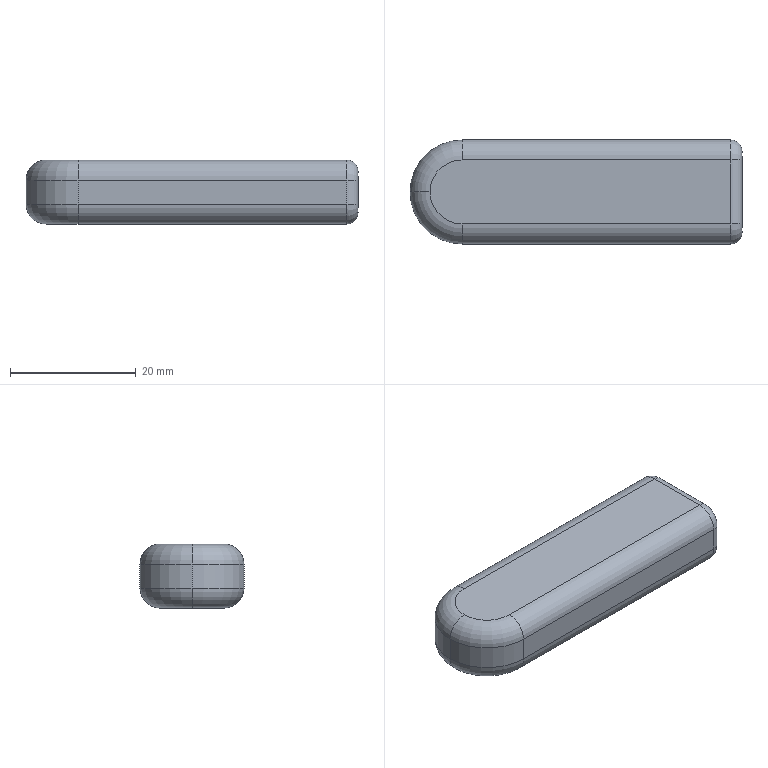Part | SolidWorks | features Fillet 3, Extrusion 1, Shell 1 | 1 solid | 32 faces | box 52.705 x 16.51 x 10.16 mm | volume 4039 mm3 | plane 12 | cylinder 12 | torus 8 | commonest cylinder face diameters 3.556 x4 6.35 x4 12.7 x2 16.51 x2
STEP:
#1=CARTESIAN_POINT('',(2.,0.05,-0.005));
#2=VERTEX_POINT('',#1);
#3=CARTESIAN_POINT('',(2.,0.45,-0.005));
#4=VERTEX_POINT('',#3);
#5=CARTESIAN_POINT('',(2.,0.5,-0.005));
#6=DIRECTION('',(0.,1.,0.));
#7=VECTOR('',#6,39.37);
#8=LINE('',#5,#7);
#9=EDGE_CURVE('',#2,#4,#8,.T.);
#10=ORIENTED_EDGE('',*,*,#9,.T.);
#11=CARTESIAN_POINT('',(2.,0.4729,0.));
#12=VERTEX_POINT('',#11);
#13=CARTESIAN_POINT('',(2.,0.45,0.05));
#14=DIRECTION('',(1.,0.,0.));
#15=DIRECTION('',(0.,0.,-1.));
#16=AXIS2_PLACEMENT_3D('',#13,#14,#15);
#17=CIRCLE('',#16,0.055);
#18=EDGE_CURVE('',#4,#12,#17,.T.);
#19=ORIENTED_EDGE('',*,*,#18,.T.);
#20=CARTESIAN_POINT('',(2.,0.02709,0.));
#21=VERTEX_POINT('',#20);
#22=CARTESIAN_POINT('',(2.,0.5,0.));
#23=DIRECTION('',(0.,-1.,0.));
#24=VECTOR('',#23,39.37);
#25=LINE('',#22,#24);
#26=EDGE_CURVE('',#12,#21,#25,.T.);
#27=ORIENTED_EDGE('',*,*,#26,.T.);
#28=CARTESIAN_POINT('',(2.,0.05,0.05));
#29=DIRECTION('',(1.,0.,0.));
#30=DIRECTION('',(0.,0.,-1.));
#31=AXIS2_PLACEMENT_3D('',#28,#29,#30);
#32=CIRCLE('',#31,0.055);
#33=EDGE_CURVE('',#21,#2,#32,.T.);
#34=ORIENTED_EDGE('',*,*,#33,.T.);
#35=EDGE_LOOP('',(#10,#19,#27,#34));
#36=FACE_OUTER_BOUND('',#35,.T.);
#37=CARTESIAN_POINT('',(2.,0.5,0.25));
#38=DIRECTION('',(1.,0.,0.));
#39=DIRECTION('',(0.,0.,-1.));
#40=AXIS2_PLACEMENT_3D('',#37,#38,#39);
#41=PLANE('',#40);
#42=ADVANCED_FACE('',(#36),#41,.T.);
#43=CARTESIAN_POINT('',(2.,0.5,0.2229));
#44=VERTEX_POINT('',#43);
#45=CARTESIAN_POINT('',(2.,0.5,0.02709));
#46=VERTEX_POINT('',#45);
#47=CARTESIAN_POINT('',(2.,0.5,0.25));
#48=DIRECTION('',(0.,0.,-1.));
#49=VECTOR('',#48,39.37);
#50=LINE('',#47,#49);
#51=EDGE_CURVE('',#44,#46,#50,.T.);
#52=ORIENTED_EDGE('',*,*,#51,.T.);
#53=CARTESIAN_POINT('',(2.,0.505,0.05));
#54=VERTEX_POINT('',#53);
#55=CARTESIAN_POINT('',(2.,0.45,0.05));
#56=DIRECTION('',(1.,0.,0.));
#57=DIRECTION('',(0.,0.,-1.));
#58=AXIS2_PLACEMENT_3D('',#55,#56,#57);
#59=CIRCLE('',#58,0.055);
#60=EDGE_CURVE('',#46,#54,#59,.T.);
#61=ORIENTED_EDGE('',*,*,#60,.T.);
#62=CARTESIAN_POINT('',(2.,0.505,0.2));
#63=VERTEX_POINT('',#62);
#64=CARTESIAN_POINT('',(2.,0.505,0.2));
#65=DIRECTION('',(0.,0.,1.));
#66=VECTOR('',#65,39.37);
#67=LINE('',#64,#66);
#68=EDGE_CURVE('',#54,#63,#67,.T.);
#69=ORIENTED_EDGE('',*,*,#68,.T.);
#70=CARTESIAN_POINT('',(2.,0.45,0.2));
#71=DIRECTION('',(1.,0.,0.));
#72=DIRECTION('',(0.,0.,-1.));
#73=AXIS2_PLACEMENT_3D('',#70,#71,#72);
#74=CIRCLE('',#73,0.055);
#75=EDGE_CURVE('',#63,#44,#74,.T.);
#76=ORIENTED_EDGE('',*,*,#75,.T.);
#77=EDGE_LOOP('',(#52,#61,#69,#76));
#78=FACE_OUTER_BOUND('',#77,.T.);
#79=CARTESIAN_POINT('',(2.,0.5,0.25));
#80=DIRECTION('',(1.,0.,0.));
#81=DIRECTION('',(0.,0.,-1.));
#82=AXIS2_PLACEMENT_3D('',#79,#80,#81);
#83=PLANE('',#82);
#84=ADVANCED_FACE('',(#78),#83,.T.);
#85=CARTESIAN_POINT('',(2.,-0.005,0.2));
#86=VERTEX_POINT('',#85);
#87=CARTESIAN_POINT('',(2.,-0.005,0.05));
#88=VERTEX_POINT('',#87);
#89=CARTESIAN_POINT('',(2.,-0.005,0.05));
#90=DIRECTION('',(0.,0.,-1.));
#91=VECTOR('',#90,39.37);
#92=LINE('',#89,#91);
#93=EDGE_CURVE('',#86,#88,#92,.T.);
#94=ORIENTED_EDGE('',*,*,#93,.T.);
#95=CARTESIAN_POINT('',(2.,0.,0.02709));
#96=VERTEX_POINT('',#95);
#97=CARTESIAN_POINT('',(2.,0.05,0.05));
#98=DIRECTION('',(1.,0.,0.));
#99=DIRECTION('',(0.,0.,-1.));
#100=AXIS2_PLACEMENT_3D('',#97,#98,#99);
#101=CIRCLE('',#100,0.055);
#102=EDGE_CURVE('',#88,#96,#101,.T.);
#103=ORIENTED_EDGE('',*,*,#102,.T.);
#104=CARTESIAN_POINT('',(2.,0.,0.2229));
#105=VERTEX_POINT('',#104);
#106=CARTESIAN_POINT('',(2.,0.,0.25));
#107=DIRECTION('',(0.,0.,-1.));
#108=VECTOR('',#107,39.37);
#109=LINE('',#106,#108);
#110=EDGE_CURVE('',#105,#96,#109,.T.);
#111=ORIENTED_EDGE('',*,*,#110,.F.);
#112=CARTESIAN_POINT('',(2.,0.05,0.2));
#113=DIRECTION('',(1.,0.,0.));
#114=DIRECTION('',(0.,0.,-1.));
#115=AXIS2_PLACEMENT_3D('',#112,#113,#114);
#116=CIRCLE('',#115,0.055);
#117=EDGE_CURVE('',#105,#86,#116,.T.);
#118=ORIENTED_EDGE('',*,*,#117,.T.);
#119=EDGE_LOOP('',(#94,#103,#111,#118));
#120=FACE_OUTER_BOUND('',#119,.T.);
#121=CARTESIAN_POINT('',(2.,0.5,0.25));
#122=DIRECTION('',(1.,0.,0.));
#123=DIRECTION('',(0.,0.,-1.));
#124=AXIS2_PLACEMENT_3D('',#121,#122,#123);
#125=PLANE('',#124);
#126=ADVANCED_FACE('',(#120),#125,.T.);
#127=CARTESIAN_POINT('',(2.,0.4729,0.25));
#128=VERTEX_POINT('',#127);
#129=CARTESIAN_POINT('',(2.,0.02709,0.25));
#130=VERTEX_POINT('',#129);
#131=CARTESIAN_POINT('',(2.,0.5,0.25));
#132=DIRECTION('',(0.,-1.,0.));
#133=VECTOR('',#132,39.37);
#134=LINE('',#131,#133);
#135=EDGE_CURVE('',#128,#130,#134,.T.);
#136=ORIENTED_EDGE('',*,*,#135,.F.);
#137=CARTESIAN_POINT('',(2.,0.45,0.255));
#138=VERTEX_POINT('',#137);
#139=CARTESIAN_POINT('',(2.,0.45,0.2));
#140=DIRECTION('',(1.,0.,0.));
#141=DIRECTION('',(0.,0.,-1.));
#142=AXIS2_PLACEMENT_3D('',#139,#140,#141);
#143=CIRCLE('',#142,0.055);
#144=EDGE_CURVE('',#128,#138,#143,.T.);
#145=ORIENTED_EDGE('',*,*,#144,.T.);
#146=CARTESIAN_POINT('',(2.,0.05,0.255));
#147=VERTEX_POINT('',#146);
#148=CARTESIAN_POINT('',(2.,0.05,0.255));
#149=DIRECTION('',(0.,-1.,0.));
#150=VECTOR('',#149,39.37);
#151=LINE('',#148,#150);
#152=EDGE_CURVE('',#138,#147,#151,.T.);
#153=ORIENTED_EDGE('',*,*,#152,.T.);
#154=CARTESIAN_POINT('',(2.,0.05,0.2));
#155=DIRECTION('',(1.,0.,0.));
#156=DIRECTION('',(0.,0.,-1.));
#157=AXIS2_PLACEMENT_3D('',#154,#155,#156);
#158=CIRCLE('',#157,0.055);
#159=EDGE_CURVE('',#147,#130,#158,.T.);
#160=ORIENTED_EDGE('',*,*,#159,.T.);
#161=EDGE_LOOP('',(#136,#145,#153,#160));
#162=FACE_OUTER_BOUND('',#161,.T.);
#163=CARTESIAN_POINT('',(2.,0.5,0.25));
#164=DIRECTION('',(1.,0.,0.));
#165=DIRECTION('',(0.,0.,-1.));
#166=AXIS2_PLACEMENT_3D('',#163,#164,#165);
#167=PLANE('',#166);
#168=ADVANCED_FACE('',(#162),#167,.T.);
#169=CARTESIAN_POINT('',(0.25,-0.075,0.05));
#170=VERTEX_POINT('',#169);
#171=CARTESIAN_POINT('',(1.93,-0.075,0.05));
#172=VERTEX_POINT('',#171);
#173=CARTESIAN_POINT('',(2.,-0.075,0.05));
#174=DIRECTION('',(1.,0.,0.));
#175=VECTOR('',#174,39.37);
#176=LINE('',#173,#175);
#177=EDGE_CURVE('',#170,#172,#176,.T.);
#178=ORIENTED_EDGE('',*,*,#177,.T.);
#179=CARTESIAN_POINT('',(1.93,-0.075,0.2));
#180=VERTEX_POINT('',#179);
#181=CARTESIAN_POINT('',(1.93,-0.075,0.2));
#182=DIRECTION('',(0.,0.,1.));
#183=VECTOR('',#182,39.37);
#184=LINE('',#181,#183);
#185=EDGE_CURVE('',#172,#180,#184,.T.);
#186=ORIENTED_EDGE('',*,*,#185,.T.);
#187=CARTESIAN_POINT('',(0.25,-0.075,0.2));
#188=VERTEX_POINT('',#187);
#189=CARTESIAN_POINT('',(0.,-0.075,0.2));
#190=DIRECTION('',(-1.,0.,0.));
#191=VECTOR('',#190,39.37);
#192=LINE('',#189,#191);
#193=EDGE_CURVE('',#180,#188,#192,.T.);
#194=ORIENTED_EDGE('',*,*,#193,.T.);
#195=CARTESIAN_POINT('',(0.25,-0.075,0.25));
#196=DIRECTION('',(0.,0.,-1.));
#197=VECTOR('',#196,39.37);
#198=LINE('',#195,#197);
#199=EDGE_CURVE('',#188,#170,#198,.T.);
#200=ORIENTED_EDGE('',*,*,#199,.T.);
#201=EDGE_LOOP('',(#178,#186,#194,#200));
#202=FACE_OUTER_BOUND('',#201,.T.);
#203=CARTESIAN_POINT('',(0.,-0.075,0.25));
#204=DIRECTION('',(0.,1.,0.));
#205=DIRECTION('',(0.,0.,1.));
#206=AXIS2_PLACEMENT_3D('',#203,#204,#205);
#207=PLANE('',#206);
#208=ADVANCED_FACE('',(#202),#207,.F.);
#209=CARTESIAN_POINT('',(0.25,0.575,0.2));
#210=VERTEX_POINT('',#209);
#211=CARTESIAN_POINT('',(1.93,0.575,0.2));
#212=VERTEX_POINT('',#211);
#213=CARTESIAN_POINT('',(2.,0.575,0.2));
#214=DIRECTION('',(1.,0.,0.));
#215=VECTOR('',#214,39.37);
#216=LINE('',#213,#215);
#217=EDGE_CURVE('',#210,#212,#216,.T.);
#218=ORIENTED_EDGE('',*,*,#217,.T.);
#219=CARTESIAN_POINT('',(1.93,0.575,0.05));
#220=VERTEX_POINT('',#219);
#221=CARTESIAN_POINT('',(1.93,0.575,0.05));
#222=DIRECTION('',(0.,0.,-1.));
#223=VECTOR('',#222,39.37);
#224=LINE('',#221,#223);
#225=EDGE_CURVE('',#212,#220,#224,.T.);
#226=ORIENTED_EDGE('',*,*,#225,.T.);
#227=CARTESIAN_POINT('',(0.25,0.575,0.05));
#228=VERTEX_POINT('',#227);
#229=CARTESIAN_POINT('',(0.25,0.575,0.05));
#230=DIRECTION('',(-1.,0.,0.));
#231=VECTOR('',#230,39.37);
#232=LINE('',#229,#231);
#233=EDGE_CURVE('',#220,#228,#232,.T.);
#234=ORIENTED_EDGE('',*,*,#233,.T.);
#235=CARTESIAN_POINT('',(0.25,0.575,0.25));
#236=DIRECTION('',(0.,0.,1.));
#237=VECTOR('',#236,39.37);
#238=LINE('',#235,#237);
#239=EDGE_CURVE('',#228,#210,#238,.T.);
#240=ORIENTED_EDGE('',*,*,#239,.T.);
#241=EDGE_LOOP('',(#218,#226,#234,#240));
#242=FACE_OUTER_BOUND('',#241,.T.);
#243=CARTESIAN_POINT('',(2.,0.575,0.25));
#244=DIRECTION('',(0.,-1.,0.));
#245=DIRECTION('',(1.,0.,0.));
#246=AXIS2_PLACEMENT_3D('',#243,#244,#245);
#247=PLANE('',#246);
#248=ADVANCED_FACE('',(#242),#247,.F.);
#249=CARTESIAN_POINT('',(0.25,0.05,0.325));
#250=VERTEX_POINT('',#249);
#251=CARTESIAN_POINT('',(1.93,0.05,0.325));
#252=VERTEX_POINT('',#251);
#253=CARTESIAN_POINT('',(0.,0.05,0.325));
#254=DIRECTION('',(1.,0.,0.));
#255=VECTOR('',#254,39.37);
#256=LINE('',#253,#255);
#257=EDGE_CURVE('',#250,#252,#256,.T.);
#258=ORIENTED_EDGE('',*,*,#257,.T.);
#259=CARTESIAN_POINT('',(1.93,0.45,0.325));
#260=VERTEX_POINT('',#259);
#261=CARTESIAN_POINT('',(1.93,0.45,0.325));
#262=DIRECTION('',(0.,1.,0.));
#263=VECTOR('',#262,39.37);
#264=LINE('',#261,#263);
#265=EDGE_CURVE('',#252,#260,#264,.T.);
#266=ORIENTED_EDGE('',*,*,#265,.T.);
#267=CARTESIAN_POINT('',(0.25,0.45,0.325));
#268=VERTEX_POINT('',#267);
#269=CARTESIAN_POINT('',(0.,0.45,0.325));
#270=DIRECTION('',(-1.,0.,0.));
#271=VECTOR('',#270,39.37);
#272=LINE('',#269,#271);
#273=EDGE_CURVE('',#260,#268,#272,.T.);
#274=ORIENTED_EDGE('',*,*,#273,.T.);
#275=CARTESIAN_POINT('',(0.05,0.25,0.325));
#276=VERTEX_POINT('',#275);
#277=CARTESIAN_POINT('',(0.25,0.25,0.325));
#278=DIRECTION('',(0.,0.,1.));
#279=DIRECTION('',(-1.,0.,0.));
#280=AXIS2_PLACEMENT_3D('',#277,#278,#279);
#281=CIRCLE('',#280,0.2);
#282=EDGE_CURVE('',#268,#276,#281,.T.);
#283=ORIENTED_EDGE('',*,*,#282,.T.);
#284=CARTESIAN_POINT('',(0.25,0.25,0.325));
#285=DIRECTION('',(0.,0.,1.));
#286=DIRECTION('',(-1.,0.,0.));
#287=AXIS2_PLACEMENT_3D('',#284,#285,#286);
#288=CIRCLE('',#287,0.2);
#289=EDGE_CURVE('',#276,#250,#288,.T.);
#290=ORIENTED_EDGE('',*,*,#289,.T.);
#291=EDGE_LOOP('',(#258,#266,#274,#283,#290));
#292=FACE_OUTER_BOUND('',#291,.T.);
#293=CARTESIAN_POINT('',(0.,0.,0.325));
#294=DIRECTION('',(0.,0.,-1.));
#295=DIRECTION('',(-1.,0.,0.));
#296=AXIS2_PLACEMENT_3D('',#293,#294,#295);
#297=PLANE('',#296);
#298=ADVANCED_FACE('',(#292),#297,.F.);
#299=CARTESIAN_POINT('',(0.25,0.45,-0.075));
#300=VERTEX_POINT('',#299);
#301=CARTESIAN_POINT('',(1.93,0.45,-0.075));
#302=VERTEX_POINT('',#301);
#303=CARTESIAN_POINT('',(2.,0.45,-0.075));
#304=DIRECTION('',(1.,0.,0.));
#305=VECTOR('',#304,39.37);
#306=LINE('',#303,#305);
#307=EDGE_CURVE('',#300,#302,#306,.T.);
#308=ORIENTED_EDGE('',*,*,#307,.T.);
#309=CARTESIAN_POINT('',(1.93,0.05,-0.075));
#310=VERTEX_POINT('',#309);
#311=CARTESIAN_POINT('',(1.93,0.,-0.075));
#312=DIRECTION('',(0.,-1.,0.));
#313=VECTOR('',#312,39.37);
#314=LINE('',#311,#313);
#315=EDGE_CURVE('',#302,#310,#314,.T.);
#316=ORIENTED_EDGE('',*,*,#315,.T.);
#317=CARTESIAN_POINT('',(0.25,0.05,-0.075));
#318=VERTEX_POINT('',#317);
#319=CARTESIAN_POINT('',(0.25,0.05,-0.075));
#320=DIRECTION('',(-1.,0.,0.));
#321=VECTOR('',#320,39.37);
#322=LINE('',#319,#321);
#323=EDGE_CURVE('',#310,#318,#322,.T.);
#324=ORIENTED_EDGE('',*,*,#323,.T.);
#325=CARTESIAN_POINT('',(0.05,0.25,-0.075));
#326=VERTEX_POINT('',#325);
#327=CARTESIAN_POINT('',(0.25,0.25,-0.075));
#328=DIRECTION('',(0.,0.,-1.));
#329=DIRECTION('',(-1.,0.,0.));
#330=AXIS2_PLACEMENT_3D('',#327,#328,#329);
#331=CIRCLE('',#330,0.2);
#332=EDGE_CURVE('',#318,#326,#331,.T.);
#333=ORIENTED_EDGE('',*,*,#332,.T.);
#334=CARTESIAN_POINT('',(0.25,0.25,-0.075));
#335=DIRECTION('',(0.,0.,-1.));
#336=DIRECTION('',(-1.,0.,0.));
#337=AXIS2_PLACEMENT_3D('',#334,#335,#336);
#338=CIRCLE('',#337,0.2);
#339=EDGE_CURVE('',#326,#300,#338,.T.);
#340=ORIENTED_EDGE('',*,*,#339,.T.);
#341=EDGE_LOOP('',(#308,#316,#324,#333,#340));
#342=FACE_OUTER_BOUND('',#341,.T.);
#343=CARTESIAN_POINT('',(0.,0.,-0.075));
#344=DIRECTION('',(0.,0.,-1.));
#345=DIRECTION('',(-1.,0.,0.));
#346=AXIS2_PLACEMENT_3D('',#343,#344,#345);
#347=PLANE('',#346);
#348=ADVANCED_FACE('',(#342),#347,.T.);
#349=CARTESIAN_POINT('',(-0.075,0.25,0.05));
#350=VERTEX_POINT('',#349);
#351=CARTESIAN_POINT('',(-0.075,0.25,0.2));
#352=VERTEX_POINT('',#351);
#353=CARTESIAN_POINT('',(-0.075,0.25,0.25));
#354=DIRECTION('',(0.,0.,1.));
#355=VECTOR('',#354,39.37);
#356=LINE('',#353,#355);
#357=EDGE_CURVE('',#350,#352,#356,.T.);
#358=ORIENTED_EDGE('',*,*,#357,.F.);
#359=CARTESIAN_POINT('',(0.25,0.25,0.05));
#360=DIRECTION('',(0.,0.,1.));
#361=DIRECTION('',(-1.,0.,0.));
#362=AXIS2_PLACEMENT_3D('',#359,#360,#361);
#363=CIRCLE('',#362,0.325);
#364=EDGE_CURVE('',#350,#170,#363,.T.);
#365=ORIENTED_EDGE('',*,*,#364,.T.);
#366=ORIENTED_EDGE('',*,*,#199,.F.);
#367=CARTESIAN_POINT('',(0.25,0.25,0.2));
#368=DIRECTION('',(0.,0.,-1.));
#369=DIRECTION('',(-1.,0.,0.));
#370=AXIS2_PLACEMENT_3D('',#367,#368,#369);
#371=CIRCLE('',#370,0.325);
#372=EDGE_CURVE('',#188,#352,#371,.T.);
#373=ORIENTED_EDGE('',*,*,#372,.T.);
#374=EDGE_LOOP('',(#358,#365,#366,#373));
#375=FACE_OUTER_BOUND('',#374,.T.);
#376=CARTESIAN_POINT('',(0.25,0.25,0.25));
#377=DIRECTION('',(0.,0.,1.));
#378=DIRECTION('',(1.,0.,0.));
#379=AXIS2_PLACEMENT_3D('',#376,#377,#378);
#380=CYLINDRICAL_SURFACE('',#379,0.325);
#381=ADVANCED_FACE('',(#375),#380,.T.);
#382=ORIENTED_EDGE('',*,*,#239,.F.);
#383=CARTESIAN_POINT('',(0.25,0.25,0.05));
#384=DIRECTION('',(0.,0.,1.));
#385=DIRECTION('',(-1.,0.,0.));
#386=AXIS2_PLACEMENT_3D('',#383,#384,#385);
#387=CIRCLE('',#386,0.325);
#388=EDGE_CURVE('',#228,#350,#387,.T.);
#389=ORIENTED_EDGE('',*,*,#388,.T.);
#390=ORIENTED_EDGE('',*,*,#357,.T.);
#391=CARTESIAN_POINT('',(0.25,0.25,0.2));
#392=DIRECTION('',(0.,0.,-1.));
#393=DIRECTION('',(-1.,0.,0.));
#394=AXIS2_PLACEMENT_3D('',#391,#392,#393);
#395=CIRCLE('',#394,0.325);
#396=EDGE_CURVE('',#352,#210,#395,.T.);
#397=ORIENTED_EDGE('',*,*,#396,.T.);
#398=EDGE_LOOP('',(#382,#389,#390,#397));
#399=FACE_OUTER_BOUND('',#398,.T.);
#400=CARTESIAN_POINT('',(0.25,0.25,0.25));
#401=DIRECTION('',(0.,0.,1.));
#402=DIRECTION('',(1.,0.,0.));
#403=AXIS2_PLACEMENT_3D('',#400,#401,#402);
#404=CYLINDRICAL_SURFACE('',#403,0.325);
#405=ADVANCED_FACE('',(#399),#404,.T.);
#406=ORIENTED_EDGE('',*,*,#110,.T.);
#407=CARTESIAN_POINT('',(1.998,0.,0.));
#408=VERTEX_POINT('',#407);
#409=CARTESIAN_POINT('',(2.,0.,0.02709));
#410=CARTESIAN_POINT('',(2.,0.,0.01802));
#411=CARTESIAN_POINT('',(2.,0.,0.008972));
#412=CARTESIAN_POINT('',(1.998,0.,0.));
#413=B_SPLINE_CURVE_WITH_KNOTS('',3,(#409,#410,#411,#412),.UNSPECIFIED.,.F.,.F.,(4,4),(0.,0.0006895),.UNSPECIFIED.);
#414=EDGE_CURVE('',#96,#408,#413,.T.);
#415=ORIENTED_EDGE('',*,*,#414,.T.);
#416=CARTESIAN_POINT('',(0.25,0.,0.));
#417=VERTEX_POINT('',#416);
#418=CARTESIAN_POINT('',(0.,0.,0.));
#419=DIRECTION('',(1.,0.,0.));
#420=VECTOR('',#419,39.37);
#421=LINE('',#418,#420);
#422=EDGE_CURVE('',#417,#408,#421,.T.);
#423=ORIENTED_EDGE('',*,*,#422,.F.);
#424=CARTESIAN_POINT('',(0.25,0.,0.25));
#425=VERTEX_POINT('',#424);
#426=CARTESIAN_POINT('',(0.25,0.,0.));
#427=DIRECTION('',(0.,0.,-1.));
#428=VECTOR('',#427,39.37);
#429=LINE('',#426,#428);
#430=EDGE_CURVE('',#425,#417,#429,.T.);
#431=ORIENTED_EDGE('',*,*,#430,.F.);
#432=CARTESIAN_POINT('',(1.998,0.,0.25));
#433=VERTEX_POINT('',#432);
#434=CARTESIAN_POINT('',(0.,0.,0.25));
#435=DIRECTION('',(1.,0.,0.));
#436=VECTOR('',#435,39.37);
#437=LINE('',#434,#436);
#438=EDGE_CURVE('',#425,#433,#437,.T.);
#439=ORIENTED_EDGE('',*,*,#438,.T.);
#440=CARTESIAN_POINT('',(1.998,0.,0.25));
#441=CARTESIAN_POINT('',(2.,0.,0.241));
#442=CARTESIAN_POINT('',(2.,0.,0.232));
#443=CARTESIAN_POINT('',(2.,0.,0.2229));
#444=B_SPLINE_CURVE_WITH_KNOTS('',3,(#440,#441,#442,#443),.UNSPECIFIED.,.F.,.F.,(4,4),(0.,0.0006895),.UNSPECIFIED.);
#445=EDGE_CURVE('',#433,#105,#444,.T.);
#446=ORIENTED_EDGE('',*,*,#445,.T.);
#447=EDGE_LOOP('',(#406,#415,#423,#431,#439,#446));
#448=FACE_OUTER_BOUND('',#447,.T.);
#449=CARTESIAN_POINT('',(0.,0.,0.25));
#450=DIRECTION('',(0.,1.,0.));
#451=DIRECTION('',(0.,0.,1.));
#452=AXIS2_PLACEMENT_3D('',#449,#450,#451);
#453=PLANE('',#452);
#454=ADVANCED_FACE('',(#448),#453,.T.);
#455=CARTESIAN_POINT('',(1.998,0.5,0.));
#456=VERTEX_POINT('',#455);
#457=CARTESIAN_POINT('',(0.25,0.5,0.));
#458=VERTEX_POINT('',#457);
#459=CARTESIAN_POINT('',(2.,0.5,0.));
#460=DIRECTION('',(-1.,0.,0.));
#461=VECTOR('',#460,39.37);
#462=LINE('',#459,#461);
#463=EDGE_CURVE('',#456,#458,#462,.T.);
#464=ORIENTED_EDGE('',*,*,#463,.F.);
#465=CARTESIAN_POINT('',(1.998,0.5,0.));
#466=CARTESIAN_POINT('',(2.,0.5,0.008972));
#467=CARTESIAN_POINT('',(2.,0.5,0.01802));
#468=CARTESIAN_POINT('',(2.,0.5,0.02709));
#469=B_SPLINE_CURVE_WITH_KNOTS('',3,(#465,#466,#467,#468),.UNSPECIFIED.,.F.,.F.,(4,4),(0.,0.0006895),.UNSPECIFIED.);
#470=EDGE_CURVE('',#456,#46,#469,.T.);
#471=ORIENTED_EDGE('',*,*,#470,.T.);
#472=ORIENTED_EDGE('',*,*,#51,.F.);
#473=CARTESIAN_POINT('',(1.998,0.5,0.25));
#474=VERTEX_POINT('',#473);
#475=CARTESIAN_POINT('',(2.,0.5,0.2229));
#476=CARTESIAN_POINT('',(2.,0.5,0.232));
#477=CARTESIAN_POINT('',(2.,0.5,0.241));
#478=CARTESIAN_POINT('',(1.998,0.5,0.25));
#479=B_SPLINE_CURVE_WITH_KNOTS('',3,(#475,#476,#477,#478),.UNSPECIFIED.,.F.,.F.,(4,4),(0.,0.0006895),.UNSPECIFIED.);
#480=EDGE_CURVE('',#44,#474,#479,.T.);
#481=ORIENTED_EDGE('',*,*,#480,.T.);
#482=CARTESIAN_POINT('',(0.25,0.5,0.25));
#483=VERTEX_POINT('',#482);
#484=CARTESIAN_POINT('',(2.,0.5,0.25));
#485=DIRECTION('',(-1.,0.,0.));
#486=VECTOR('',#485,39.37);
#487=LINE('',#484,#486);
#488=EDGE_CURVE('',#474,#483,#487,.T.);
#489=ORIENTED_EDGE('',*,*,#488,.T.);
#490=CARTESIAN_POINT('',(0.25,0.5,0.25));
#491=DIRECTION('',(0.,0.,1.));
#492=VECTOR('',#491,39.37);
#493=LINE('',#490,#492);
#494=EDGE_CURVE('',#458,#483,#493,.T.);
#495=ORIENTED_EDGE('',*,*,#494,.F.);
#496=EDGE_LOOP('',(#464,#471,#472,#481,#489,#495));
#497=FACE_OUTER_BOUND('',#496,.T.);
#498=CARTESIAN_POINT('',(2.,0.5,0.25));
#499=DIRECTION('',(0.,-1.,0.));
#500=DIRECTION('',(1.,0.,0.));
#501=AXIS2_PLACEMENT_3D('',#498,#499,#500);
#502=PLANE('',#501);
#503=ADVANCED_FACE('',(#497),#502,.T.);
#504=ORIENTED_EDGE('',*,*,#488,.F.);
#505=CARTESIAN_POINT('',(1.998,0.5,0.25));
#506=CARTESIAN_POINT('',(2.,0.491,0.25));
#507=CARTESIAN_POINT('',(2.,0.482,0.25));
#508=CARTESIAN_POINT('',(2.,0.4729,0.25));
#509=B_SPLINE_CURVE_WITH_KNOTS('',3,(#505,#506,#507,#508),.UNSPECIFIED.,.F.,.F.,(4,4),(0.,0.0006895),.UNSPECIFIED.);
#510=EDGE_CURVE('',#474,#128,#509,.T.);
#511=ORIENTED_EDGE('',*,*,#510,.T.);
#512=ORIENTED_EDGE('',*,*,#135,.T.);
#513=CARTESIAN_POINT('',(2.,0.02709,0.25));
#514=CARTESIAN_POINT('',(2.,0.01802,0.25));
#515=CARTESIAN_POINT('',(2.,0.008972,0.25));
#516=CARTESIAN_POINT('',(1.998,0.,0.25));
#517=B_SPLINE_CURVE_WITH_KNOTS('',3,(#513,#514,#515,#516),.UNSPECIFIED.,.F.,.F.,(4,4),(0.,0.0006895),.UNSPECIFIED.);
#518=EDGE_CURVE('',#130,#433,#517,.T.);
#519=ORIENTED_EDGE('',*,*,#518,.T.);
#520=ORIENTED_EDGE('',*,*,#438,.F.);
#521=CARTESIAN_POINT('',(0.,0.25,0.25));
#522=VERTEX_POINT('',#521);
#523=CARTESIAN_POINT('',(0.25,0.25,0.25));
#524=DIRECTION('',(0.,0.,1.));
#525=DIRECTION('',(-1.,0.,0.));
#526=AXIS2_PLACEMENT_3D('',#523,#524,#525);
#527=CIRCLE('',#526,0.25);
#528=EDGE_CURVE('',#522,#425,#527,.T.);
#529=ORIENTED_EDGE('',*,*,#528,.F.);
#530=CARTESIAN_POINT('',(0.25,0.25,0.25));
#531=DIRECTION('',(0.,0.,1.));
#532=DIRECTION('',(-1.,0.,0.));
#533=AXIS2_PLACEMENT_3D('',#530,#531,#532);
#534=CIRCLE('',#533,0.25);
#535=EDGE_CURVE('',#483,#522,#534,.T.);
#536=ORIENTED_EDGE('',*,*,#535,.F.);
#537=EDGE_LOOP('',(#504,#511,#512,#519,#520,#529,#536));
#538=FACE_OUTER_BOUND('',#537,.T.);
#539=CARTESIAN_POINT('',(0.,0.,0.25));
#540=DIRECTION('',(0.,0.,-1.));
#541=DIRECTION('',(-1.,0.,0.));
#542=AXIS2_PLACEMENT_3D('',#539,#540,#541);
#543=PLANE('',#542);
#544=ADVANCED_FACE('',(#538),#543,.T.);
#545=ORIENTED_EDGE('',*,*,#26,.F.);
#546=CARTESIAN_POINT('',(2.,0.4729,0.));
#547=CARTESIAN_POINT('',(2.,0.482,0.));
#548=CARTESIAN_POINT('',(2.,0.491,0.));
#549=CARTESIAN_POINT('',(1.998,0.5,0.));
#550=B_SPLINE_CURVE_WITH_KNOTS('',3,(#546,#547,#548,#549),.UNSPECIFIED.,.F.,.F.,(4,4),(0.,0.0006895),.UNSPECIFIED.);
#551=EDGE_CURVE('',#12,#456,#550,.T.);
#552=ORIENTED_EDGE('',*,*,#551,.T.);
#553=ORIENTED_EDGE('',*,*,#463,.T.);
#554=CARTESIAN_POINT('',(0.,0.25,0.));
#555=VERTEX_POINT('',#554);
#556=CARTESIAN_POINT('',(0.25,0.25,0.));
#557=DIRECTION('',(0.,0.,-1.));
#558=DIRECTION('',(-1.,0.,0.));
#559=AXIS2_PLACEMENT_3D('',#556,#557,#558);
#560=CIRCLE('',#559,0.25);
#561=EDGE_CURVE('',#555,#458,#560,.T.);
#562=ORIENTED_EDGE('',*,*,#561,.F.);
#563=CARTESIAN_POINT('',(0.25,0.25,0.));
#564=DIRECTION('',(0.,0.,-1.));
#565=DIRECTION('',(-1.,0.,0.));
#566=AXIS2_PLACEMENT_3D('',#563,#564,#565);
#567=CIRCLE('',#566,0.25);
#568=EDGE_CURVE('',#417,#555,#567,.T.);
#569=ORIENTED_EDGE('',*,*,#568,.F.);
#570=ORIENTED_EDGE('',*,*,#422,.T.);
#571=CARTESIAN_POINT('',(1.998,0.,0.));
#572=CARTESIAN_POINT('',(2.,0.008972,0.));
#573=CARTESIAN_POINT('',(2.,0.01802,0.));
#574=CARTESIAN_POINT('',(2.,0.02709,0.));
#575=B_SPLINE_CURVE_WITH_KNOTS('',3,(#571,#572,#573,#574),.UNSPECIFIED.,.F.,.F.,(4,4),(0.,0.0006895),.UNSPECIFIED.);
#576=EDGE_CURVE('',#408,#21,#575,.T.);
#577=ORIENTED_EDGE('',*,*,#576,.T.);
#578=EDGE_LOOP('',(#545,#552,#553,#562,#569,#570,#577));
#579=FACE_OUTER_BOUND('',#578,.T.);
#580=CARTESIAN_POINT('',(0.,0.,0.));
#581=DIRECTION('',(0.,0.,-1.));
#582=DIRECTION('',(-1.,0.,0.));
#583=AXIS2_PLACEMENT_3D('',#580,#581,#582);
#584=PLANE('',#583);
#585=ADVANCED_FACE('',(#579),#584,.F.);
#586=ORIENTED_EDGE('',*,*,#430,.T.);
#587=ORIENTED_EDGE('',*,*,#568,.T.);
#588=CARTESIAN_POINT('',(0.,0.25,0.25));
#589=DIRECTION('',(0.,0.,1.));
#590=VECTOR('',#589,39.37);
#591=LINE('',#588,#590);
#592=EDGE_CURVE('',#555,#522,#591,.T.);
#593=ORIENTED_EDGE('',*,*,#592,.T.);
#594=ORIENTED_EDGE('',*,*,#528,.T.);
#595=EDGE_LOOP('',(#586,#587,#593,#594));
#596=FACE_OUTER_BOUND('',#595,.T.);
#597=CARTESIAN_POINT('',(0.25,0.25,0.25));
#598=DIRECTION('',(0.,0.,1.));
#599=DIRECTION('',(1.,0.,0.));
#600=AXIS2_PLACEMENT_3D('',#597,#598,#599);
#601=CYLINDRICAL_SURFACE('',#600,0.25);
#602=ADVANCED_FACE('',(#596),#601,.F.);
#603=ORIENTED_EDGE('',*,*,#535,.T.);
#604=ORIENTED_EDGE('',*,*,#592,.F.);
#605=ORIENTED_EDGE('',*,*,#561,.T.);
#606=ORIENTED_EDGE('',*,*,#494,.T.);
#607=EDGE_LOOP('',(#603,#604,#605,#606));
#608=FACE_OUTER_BOUND('',#607,.T.);
#609=CARTESIAN_POINT('',(0.25,0.25,0.25));
#610=DIRECTION('',(0.,0.,1.));
#611=DIRECTION('',(1.,0.,0.));
#612=AXIS2_PLACEMENT_3D('',#609,#610,#611);
#613=CYLINDRICAL_SURFACE('',#612,0.25);
#614=ADVANCED_FACE('',(#608),#613,.F.);
#615=ORIENTED_EDGE('',*,*,#233,.F.);
#616=CARTESIAN_POINT('',(1.93,0.45,0.05));
#617=DIRECTION('',(-1.,0.,0.));
#618=DIRECTION('',(0.,0.,-1.));
#619=AXIS2_PLACEMENT_3D('',#616,#617,#618);
#620=CIRCLE('',#619,0.125);
#621=EDGE_CURVE('',#220,#302,#620,.T.);
#622=ORIENTED_EDGE('',*,*,#621,.T.);
#623=ORIENTED_EDGE('',*,*,#307,.F.);
#624=CARTESIAN_POINT('',(0.25,0.45,0.05));
#625=DIRECTION('',(-1.,0.,0.));
#626=DIRECTION('',(0.,0.,1.));
#627=AXIS2_PLACEMENT_3D('',#624,#625,#626);
#628=CIRCLE('',#627,0.125);
#629=EDGE_CURVE('',#228,#300,#628,.T.);
#630=ORIENTED_EDGE('',*,*,#629,.F.);
#631=EDGE_LOOP('',(#615,#622,#623,#630));
#632=FACE_OUTER_BOUND('',#631,.T.);
#633=CARTESIAN_POINT('',(2.,0.45,0.05));
#634=DIRECTION('',(1.,0.,0.));
#635=DIRECTION('',(0.,1.,0.));
#636=AXIS2_PLACEMENT_3D('',#633,#634,#635);
#637=CYLINDRICAL_SURFACE('',#636,0.125);
#638=ADVANCED_FACE('',(#632),#637,.T.);
#639=ORIENTED_EDGE('',*,*,#629,.T.);
#640=ORIENTED_EDGE('',*,*,#339,.F.);
#641=CARTESIAN_POINT('',(0.05,0.25,0.05));
#642=DIRECTION('',(0.,-1.,0.));
#643=DIRECTION('',(0.,0.,-1.));
#644=AXIS2_PLACEMENT_3D('',#641,#642,#643);
#645=CIRCLE('',#644,0.125);
#646=EDGE_CURVE('',#350,#326,#645,.T.);
#647=ORIENTED_EDGE('',*,*,#646,.F.);
#648=ORIENTED_EDGE('',*,*,#388,.F.);
#649=EDGE_LOOP('',(#639,#640,#647,#648));
#650=FACE_OUTER_BOUND('',#649,.T.);
#651=CARTESIAN_POINT('',(0.25,0.25,0.05));
#652=DIRECTION('',(0.,0.,-1.));
#653=DIRECTION('',(-1.,0.,0.));
#654=AXIS2_PLACEMENT_3D('',#651,#652,#653);
#655=TOROIDAL_SURFACE('',#654,0.2,0.125);
#656=ADVANCED_FACE('',(#650),#655,.T.);
#657=ORIENTED_EDGE('',*,*,#646,.T.);
#658=ORIENTED_EDGE('',*,*,#332,.F.);
#659=CARTESIAN_POINT('',(0.25,0.05,0.05));
#660=DIRECTION('',(1.,0.,0.));
#661=DIRECTION('',(0.,0.,-1.));
#662=AXIS2_PLACEMENT_3D('',#659,#660,#661);
#663=CIRCLE('',#662,0.125);
#664=EDGE_CURVE('',#170,#318,#663,.T.);
#665=ORIENTED_EDGE('',*,*,#664,.F.);
#666=ORIENTED_EDGE('',*,*,#364,.F.);
#667=EDGE_LOOP('',(#657,#658,#665,#666));
#668=FACE_OUTER_BOUND('',#667,.T.);
#669=CARTESIAN_POINT('',(0.25,0.25,0.05));
#670=DIRECTION('',(0.,0.,-1.));
#671=DIRECTION('',(-1.,0.,0.));
#672=AXIS2_PLACEMENT_3D('',#669,#670,#671);
#673=TOROIDAL_SURFACE('',#672,0.2,0.125);
#674=ADVANCED_FACE('',(#668),#673,.T.);
#675=ORIENTED_EDGE('',*,*,#323,.F.);
#676=CARTESIAN_POINT('',(1.93,0.05,0.05));
#677=DIRECTION('',(-1.,0.,0.));
#678=DIRECTION('',(0.,0.,-1.));
#679=AXIS2_PLACEMENT_3D('',#676,#677,#678);
#680=CIRCLE('',#679,0.125);
#681=EDGE_CURVE('',#310,#172,#680,.T.);
#682=ORIENTED_EDGE('',*,*,#681,.T.);
#683=ORIENTED_EDGE('',*,*,#177,.F.);
#684=ORIENTED_EDGE('',*,*,#664,.T.);
#685=EDGE_LOOP('',(#675,#682,#683,#684));
#686=FACE_OUTER_BOUND('',#685,.T.);
#687=CARTESIAN_POINT('',(0.,0.05,0.05));
#688=DIRECTION('',(-1.,0.,0.));
#689=DIRECTION('',(0.,0.,1.));
#690=AXIS2_PLACEMENT_3D('',#687,#688,#689);
#691=CYLINDRICAL_SURFACE('',#690,0.125);
#692=ADVANCED_FACE('',(#686),#691,.T.);
#693=ORIENTED_EDGE('',*,*,#273,.F.);
#694=CARTESIAN_POINT('',(1.93,0.45,0.2));
#695=DIRECTION('',(-1.,0.,0.));
#696=DIRECTION('',(0.,0.,-1.));
#697=AXIS2_PLACEMENT_3D('',#694,#695,#696);
#698=CIRCLE('',#697,0.125);
#699=EDGE_CURVE('',#260,#212,#698,.T.);
#700=ORIENTED_EDGE('',*,*,#699,.T.);
#701=ORIENTED_EDGE('',*,*,#217,.F.);
#702=CARTESIAN_POINT('',(0.25,0.45,0.2));
#703=DIRECTION('',(-1.,0.,0.));
#704=DIRECTION('',(0.,-1.,0.));
#705=AXIS2_PLACEMENT_3D('',#702,#703,#704);
#706=CIRCLE('',#705,0.125);
#707=EDGE_CURVE('',#268,#210,#706,.T.);
#708=ORIENTED_EDGE('',*,*,#707,.F.);
#709=EDGE_LOOP('',(#693,#700,#701,#708));
#710=FACE_OUTER_BOUND('',#709,.T.);
#711=CARTESIAN_POINT('',(0.,0.45,0.2));
#712=DIRECTION('',(-1.,0.,0.));
#713=DIRECTION('',(0.,-1.,0.));
#714=AXIS2_PLACEMENT_3D('',#711,#712,#713);
#715=CYLINDRICAL_SURFACE('',#714,0.125);
#716=ADVANCED_FACE('',(#710),#715,.T.);
#717=ORIENTED_EDGE('',*,*,#707,.T.);
#718=ORIENTED_EDGE('',*,*,#396,.F.);
#719=CARTESIAN_POINT('',(0.05,0.25,0.2));
#720=DIRECTION('',(0.,-1.,0.));
#721=DIRECTION('',(0.,0.,-1.));
#722=AXIS2_PLACEMENT_3D('',#719,#720,#721);
#723=CIRCLE('',#722,0.125);
#724=EDGE_CURVE('',#276,#352,#723,.T.);
#725=ORIENTED_EDGE('',*,*,#724,.F.);
#726=ORIENTED_EDGE('',*,*,#282,.F.);
#727=EDGE_LOOP('',(#717,#718,#725,#726));
#728=FACE_OUTER_BOUND('',#727,.T.);
#729=CARTESIAN_POINT('',(0.25,0.25,0.2));
#730=DIRECTION('',(0.,0.,-1.));
#731=DIRECTION('',(-1.,0.,0.));
#732=AXIS2_PLACEMENT_3D('',#729,#730,#731);
#733=TOROIDAL_SURFACE('',#732,0.2,0.125);
#734=ADVANCED_FACE('',(#728),#733,.T.);
#735=ORIENTED_EDGE('',*,*,#724,.T.);
#736=ORIENTED_EDGE('',*,*,#372,.F.);
#737=CARTESIAN_POINT('',(0.25,0.05,0.2));
#738=DIRECTION('',(1.,0.,0.));
#739=DIRECTION('',(0.,0.,-1.));
#740=AXIS2_PLACEMENT_3D('',#737,#738,#739);
#741=CIRCLE('',#740,0.125);
#742=EDGE_CURVE('',#250,#188,#741,.T.);
#743=ORIENTED_EDGE('',*,*,#742,.F.);
#744=ORIENTED_EDGE('',*,*,#289,.F.);
#745=EDGE_LOOP('',(#735,#736,#743,#744));
#746=FACE_OUTER_BOUND('',#745,.T.);
#747=CARTESIAN_POINT('',(0.25,0.25,0.2));
#748=DIRECTION('',(0.,0.,-1.));
#749=DIRECTION('',(-1.,0.,0.));
#750=AXIS2_PLACEMENT_3D('',#747,#748,#749);
#751=TOROIDAL_SURFACE('',#750,0.2,0.125);
#752=ADVANCED_FACE('',(#746),#751,.T.);
#753=ORIENTED_EDGE('',*,*,#193,.F.);
#754=CARTESIAN_POINT('',(1.93,0.05,0.2));
#755=DIRECTION('',(-1.,0.,0.));
#756=DIRECTION('',(0.,0.,-1.));
#757=AXIS2_PLACEMENT_3D('',#754,#755,#756);
#758=CIRCLE('',#757,0.125);
#759=EDGE_CURVE('',#180,#252,#758,.T.);
#760=ORIENTED_EDGE('',*,*,#759,.T.);
#761=ORIENTED_EDGE('',*,*,#257,.F.);
#762=ORIENTED_EDGE('',*,*,#742,.T.);
#763=EDGE_LOOP('',(#753,#760,#761,#762));
#764=FACE_OUTER_BOUND('',#763,.T.);
#765=CARTESIAN_POINT('',(0.,0.05,0.2));
#766=DIRECTION('',(1.,0.,0.));
#767=DIRECTION('',(0.,0.,-1.));
#768=AXIS2_PLACEMENT_3D('',#765,#766,#767);
#769=CYLINDRICAL_SURFACE('',#768,0.125);
#770=ADVANCED_FACE('',(#764),#769,.T.);
#771=CARTESIAN_POINT('',(1.93,0.05,0.255));
#772=DIRECTION('',(0.,-1.,0.));
#773=DIRECTION('',(0.,0.,-1.));
#774=AXIS2_PLACEMENT_3D('',#771,#772,#773);
#775=CIRCLE('',#774,0.07);
#776=EDGE_CURVE('',#147,#252,#775,.T.);
#777=ORIENTED_EDGE('',*,*,#776,.F.);
#778=ORIENTED_EDGE('',*,*,#152,.F.);
#779=CARTESIAN_POINT('',(1.93,0.45,0.255));
#780=DIRECTION('',(0.,1.,0.));
#781=DIRECTION('',(0.,0.,1.));
#782=AXIS2_PLACEMENT_3D('',#779,#780,#781);
#783=CIRCLE('',#782,0.07);
#784=EDGE_CURVE('',#260,#138,#783,.T.);
#785=ORIENTED_EDGE('',*,*,#784,.F.);
#786=ORIENTED_EDGE('',*,*,#265,.F.);
#787=EDGE_LOOP('',(#777,#778,#785,#786));
#788=FACE_OUTER_BOUND('',#787,.T.);
#789=CARTESIAN_POINT('',(1.93,0.5,0.255));
#790=DIRECTION('',(0.,1.,0.));
#791=DIRECTION('',(0.,0.,1.));
#792=AXIS2_PLACEMENT_3D('',#789,#790,#791);
#793=CYLINDRICAL_SURFACE('',#792,0.07);
#794=ADVANCED_FACE('',(#788),#793,.T.);
#795=ORIENTED_EDGE('',*,*,#480,.F.);
#796=ORIENTED_EDGE('',*,*,#75,.F.);
#797=CARTESIAN_POINT('',(1.93,0.505,0.2));
#798=DIRECTION('',(0.,0.,-1.));
#799=DIRECTION('',(-1.,0.,0.));
#800=AXIS2_PLACEMENT_3D('',#797,#798,#799);
#801=CIRCLE('',#800,0.07);
#802=EDGE_CURVE('',#212,#63,#801,.T.);
#803=ORIENTED_EDGE('',*,*,#802,.F.);
#804=ORIENTED_EDGE('',*,*,#699,.F.);
#805=ORIENTED_EDGE('',*,*,#784,.T.);
#806=ORIENTED_EDGE('',*,*,#144,.F.);
#807=ORIENTED_EDGE('',*,*,#510,.F.);
#808=EDGE_LOOP('',(#795,#796,#803,#804,#805,#806,#807));
#809=FACE_OUTER_BOUND('',#808,.T.);
#810=CARTESIAN_POINT('',(1.93,0.45,0.2));
#811=DIRECTION('',(1.,0.,0.));
#812=DIRECTION('',(0.,0.,-1.));
#813=AXIS2_PLACEMENT_3D('',#810,#811,#812);
#814=TOROIDAL_SURFACE('',#813,0.055,0.07);
#815=ADVANCED_FACE('',(#809),#814,.T.);
#816=ORIENTED_EDGE('',*,*,#776,.T.);
#817=ORIENTED_EDGE('',*,*,#759,.F.);
#818=CARTESIAN_POINT('',(1.93,-0.005,0.2));
#819=DIRECTION('',(0.,0.,-1.));
#820=DIRECTION('',(-1.,0.,0.));
#821=AXIS2_PLACEMENT_3D('',#818,#819,#820);
#822=CIRCLE('',#821,0.07);
#823=EDGE_CURVE('',#86,#180,#822,.T.);
#824=ORIENTED_EDGE('',*,*,#823,.F.);
#825=ORIENTED_EDGE('',*,*,#117,.F.);
#826=ORIENTED_EDGE('',*,*,#445,.F.);
#827=ORIENTED_EDGE('',*,*,#518,.F.);
#828=ORIENTED_EDGE('',*,*,#159,.F.);
#829=EDGE_LOOP('',(#816,#817,#824,#825,#826,#827,#828));
#830=FACE_OUTER_BOUND('',#829,.T.);
#831=CARTESIAN_POINT('',(1.93,0.05,0.2));
#832=DIRECTION('',(1.,0.,0.));
#833=DIRECTION('',(0.,0.,-1.));
#834=AXIS2_PLACEMENT_3D('',#831,#832,#833);
#835=TOROIDAL_SURFACE('',#834,0.055,0.07);
#836=ADVANCED_FACE('',(#830),#835,.T.);
#837=ORIENTED_EDGE('',*,*,#802,.T.);
#838=ORIENTED_EDGE('',*,*,#68,.F.);
#839=CARTESIAN_POINT('',(1.93,0.505,0.05));
#840=DIRECTION('',(0.,0.,-1.));
#841=DIRECTION('',(-1.,0.,0.));
#842=AXIS2_PLACEMENT_3D('',#839,#840,#841);
#843=CIRCLE('',#842,0.07);
#844=EDGE_CURVE('',#220,#54,#843,.T.);
#845=ORIENTED_EDGE('',*,*,#844,.F.);
#846=ORIENTED_EDGE('',*,*,#225,.F.);
#847=EDGE_LOOP('',(#837,#838,#845,#846));
#848=FACE_OUTER_BOUND('',#847,.T.);
#849=CARTESIAN_POINT('',(1.93,0.505,0.25));
#850=DIRECTION('',(0.,0.,1.));
#851=DIRECTION('',(1.,0.,0.));
#852=AXIS2_PLACEMENT_3D('',#849,#850,#851);
#853=CYLINDRICAL_SURFACE('',#852,0.07);
#854=ADVANCED_FACE('',(#848),#853,.T.);
#855=ORIENTED_EDGE('',*,*,#823,.T.);
#856=ORIENTED_EDGE('',*,*,#185,.F.);
#857=CARTESIAN_POINT('',(1.93,-0.005,0.05));
#858=DIRECTION('',(0.,0.,-1.));
#859=DIRECTION('',(-1.,0.,0.));
#860=AXIS2_PLACEMENT_3D('',#857,#858,#859);
#861=CIRCLE('',#860,0.07);
#862=EDGE_CURVE('',#88,#172,#861,.T.);
#863=ORIENTED_EDGE('',*,*,#862,.F.);
#864=ORIENTED_EDGE('',*,*,#93,.F.);
#865=EDGE_LOOP('',(#855,#856,#863,#864));
#866=FACE_OUTER_BOUND('',#865,.T.);
#867=CARTESIAN_POINT('',(1.93,-0.005,0.25));
#868=DIRECTION('',(0.,0.,1.));
#869=DIRECTION('',(1.,0.,0.));
#870=AXIS2_PLACEMENT_3D('',#867,#868,#869);
#871=CYLINDRICAL_SURFACE('',#870,0.07);
#872=ADVANCED_FACE('',(#866),#871,.T.);
#873=ORIENTED_EDGE('',*,*,#551,.F.);
#874=ORIENTED_EDGE('',*,*,#18,.F.);
#875=CARTESIAN_POINT('',(1.93,0.45,-0.005));
#876=DIRECTION('',(0.,-1.,0.));
#877=DIRECTION('',(0.,0.,-1.));
#878=AXIS2_PLACEMENT_3D('',#875,#876,#877);
#879=CIRCLE('',#878,0.07);
#880=EDGE_CURVE('',#302,#4,#879,.T.);
#881=ORIENTED_EDGE('',*,*,#880,.F.);
#882=ORIENTED_EDGE('',*,*,#621,.F.);
#883=ORIENTED_EDGE('',*,*,#844,.T.);
#884=ORIENTED_EDGE('',*,*,#60,.F.);
#885=ORIENTED_EDGE('',*,*,#470,.F.);
#886=EDGE_LOOP('',(#873,#874,#881,#882,#883,#884,#885));
#887=FACE_OUTER_BOUND('',#886,.T.);
#888=CARTESIAN_POINT('',(1.93,0.45,0.05));
#889=DIRECTION('',(1.,0.,0.));
#890=DIRECTION('',(0.,0.,-1.));
#891=AXIS2_PLACEMENT_3D('',#888,#889,#890);
#892=TOROIDAL_SURFACE('',#891,0.055,0.07);
#893=ADVANCED_FACE('',(#887),#892,.T.);
#894=ORIENTED_EDGE('',*,*,#862,.T.);
#895=ORIENTED_EDGE('',*,*,#681,.F.);
#896=CARTESIAN_POINT('',(1.93,0.05,-0.005));
#897=DIRECTION('',(0.,1.,0.));
#898=DIRECTION('',(0.,0.,1.));
#899=AXIS2_PLACEMENT_3D('',#896,#897,#898);
#900=CIRCLE('',#899,0.07);
#901=EDGE_CURVE('',#2,#310,#900,.T.);
#902=ORIENTED_EDGE('',*,*,#901,.F.);
#903=ORIENTED_EDGE('',*,*,#33,.F.);
#904=ORIENTED_EDGE('',*,*,#576,.F.);
#905=ORIENTED_EDGE('',*,*,#414,.F.);
#906=ORIENTED_EDGE('',*,*,#102,.F.);
#907=EDGE_LOOP('',(#894,#895,#902,#903,#904,#905,#906));
#908=FACE_OUTER_BOUND('',#907,.T.);
#909=CARTESIAN_POINT('',(1.93,0.05,0.05));
#910=DIRECTION('',(1.,0.,0.));
#911=DIRECTION('',(0.,0.,-1.));
#912=AXIS2_PLACEMENT_3D('',#909,#910,#911);
#913=TOROIDAL_SURFACE('',#912,0.055,0.07);
#914=ADVANCED_FACE('',(#908),#913,.T.);
#915=ORIENTED_EDGE('',*,*,#880,.T.);
#916=ORIENTED_EDGE('',*,*,#9,.F.);
#917=ORIENTED_EDGE('',*,*,#901,.T.);
#918=ORIENTED_EDGE('',*,*,#315,.F.);
#919=EDGE_LOOP('',(#915,#916,#917,#918));
#920=FACE_OUTER_BOUND('',#919,.T.);
#921=CARTESIAN_POINT('',(1.93,0.,-0.005));
#922=DIRECTION('',(0.,-1.,0.));
#923=DIRECTION('',(0.,0.,-1.));
#924=AXIS2_PLACEMENT_3D('',#921,#922,#923);
#925=CYLINDRICAL_SURFACE('',#924,0.07);
#926=ADVANCED_FACE('',(#920),#925,.T.);
#927=CLOSED_SHELL('',(#42,#84,#126,#168,#208,#248,#298,#348,#381,#405,#454,#503,#544,#585,#602,#614,#638,#656,#674,#692,#716,#734,#752,#770,#794,#815,#836,#854,#872,#893,#914,#926));
#928=MANIFOLD_SOLID_BREP('',#927);
#929=CARTESIAN_POINT('',(0.,0.,0.));
#930=DIRECTION('',(0.,0.,1.));
#931=DIRECTION('',(1.,0.,0.));
#932=AXIS2_PLACEMENT_3D('',#929,#930,#931);
#933=(LENGTH_UNIT()NAMED_UNIT(*)SI_UNIT($,.METRE.));
#934=LENGTH_MEASURE_WITH_UNIT(LENGTH_MEASURE(0.0254),#933);
#935=DIMENSIONAL_EXPONENTS(1.,0.,0.,0.,0.,0.,0.);
#936=(CONVERSION_BASED_UNIT('INCH',#934)LENGTH_UNIT()NAMED_UNIT(#935));
#937=UNCERTAINTY_MEASURE_WITH_UNIT(LENGTH_MEASURE(0.00001),#936,'','');
#938=(NAMED_UNIT(*)PLANE_ANGLE_UNIT()SI_UNIT($,.RADIAN.));
#939=(NAMED_UNIT(*)SI_UNIT($,.STERADIAN.)SOLID_ANGLE_UNIT());
#940=(GEOMETRIC_REPRESENTATION_CONTEXT(3)GLOBAL_UNCERTAINTY_ASSIGNED_CONTEXT((#937))GLOBAL_UNIT_ASSIGNED_CONTEXT((#936,#938,#939))REPRESENTATION_CONTEXT('',''));
#941=ADVANCED_BREP_SHAPE_REPRESENTATION('',(#928,#932),#940);